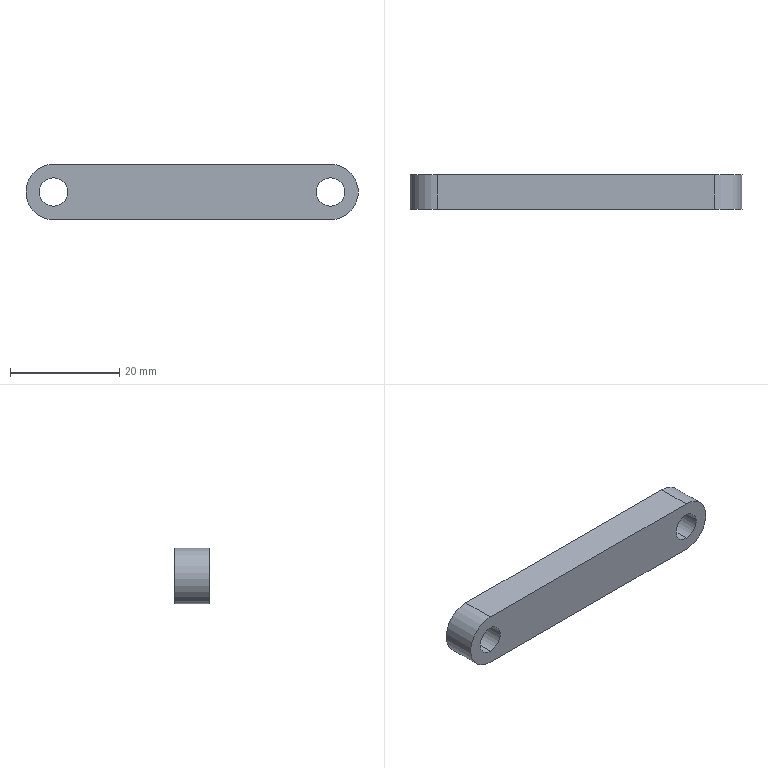Part | SolidWorks | features Extrusion 1, ICE 1 | 1 solid | 10 faces | box 60.96 x 6.35 x 10.16 mm | volume 3522 mm3 | cylinder 6 | plane 4 | commonest cylinder face diameters 5.207 x4 10.16 x2
STEP:
#1=CARTESIAN_POINT('',(50.8,0.,-2.604));
#2=VERTEX_POINT('',#1);
#3=CARTESIAN_POINT('',(50.8,0.,2.604));
#4=VERTEX_POINT('',#3);
#5=CARTESIAN_POINT('',(50.8,0.,0.));
#6=DIRECTION('',(0.,1.,0.));
#7=DIRECTION('',(0.,0.,-1.));
#8=AXIS2_PLACEMENT_3D('',#5,#6,#7);
#9=CIRCLE('',#8,2.604);
#10=EDGE_CURVE('',#2,#4,#9,.T.);
#11=ORIENTED_EDGE('',*,*,#10,.F.);
#12=CARTESIAN_POINT('',(50.8,6.35,-2.604));
#13=VERTEX_POINT('',#12);
#14=CARTESIAN_POINT('',(50.8,-8.202,-2.604));
#15=DIRECTION('',(0.,1.,0.));
#16=VECTOR('',#15,1000.);
#17=LINE('',#14,#16);
#18=EDGE_CURVE('',#2,#13,#17,.T.);
#19=ORIENTED_EDGE('',*,*,#18,.T.);
#20=CARTESIAN_POINT('',(50.8,6.35,2.604));
#21=VERTEX_POINT('',#20);
#22=CARTESIAN_POINT('',(50.8,6.35,0.));
#23=DIRECTION('',(0.,1.,0.));
#24=DIRECTION('',(0.,0.,1.));
#25=AXIS2_PLACEMENT_3D('',#22,#23,#24);
#26=CIRCLE('',#25,2.604);
#27=EDGE_CURVE('',#13,#21,#26,.T.);
#28=ORIENTED_EDGE('',*,*,#27,.T.);
#29=CARTESIAN_POINT('',(50.8,-8.202,2.604));
#30=DIRECTION('',(0.,1.,0.));
#31=VECTOR('',#30,1000.);
#32=LINE('',#29,#31);
#33=EDGE_CURVE('',#4,#21,#32,.T.);
#34=ORIENTED_EDGE('',*,*,#33,.F.);
#35=EDGE_LOOP('',(#11,#19,#28,#34));
#36=FACE_OUTER_BOUND('',#35,.T.);
#37=CARTESIAN_POINT('',(50.8,-8.202,0.));
#38=DIRECTION('',(0.,1.,0.));
#39=DIRECTION('',(0.,0.,1.));
#40=AXIS2_PLACEMENT_3D('',#37,#38,#39);
#41=CYLINDRICAL_SURFACE('',#40,2.604);
#42=ADVANCED_FACE('',(#36),#41,.F.);
#43=CARTESIAN_POINT('',(0.,0.,-2.603));
#44=VERTEX_POINT('',#43);
#45=CARTESIAN_POINT('',(0.,0.,2.603));
#46=VERTEX_POINT('',#45);
#47=CARTESIAN_POINT('',(0.,0.,0.));
#48=DIRECTION('',(0.,1.,0.));
#49=DIRECTION('',(0.,0.,-1.));
#50=AXIS2_PLACEMENT_3D('',#47,#48,#49);
#51=CIRCLE('',#50,2.603);
#52=EDGE_CURVE('',#44,#46,#51,.T.);
#53=ORIENTED_EDGE('',*,*,#52,.F.);
#54=CARTESIAN_POINT('',(0.,6.35,-2.603));
#55=VERTEX_POINT('',#54);
#56=CARTESIAN_POINT('',(0.,-8.202,-2.603));
#57=DIRECTION('',(0.,1.,0.));
#58=VECTOR('',#57,1000.);
#59=LINE('',#56,#58);
#60=EDGE_CURVE('',#44,#55,#59,.T.);
#61=ORIENTED_EDGE('',*,*,#60,.T.);
#62=CARTESIAN_POINT('',(0.,6.35,2.603));
#63=VERTEX_POINT('',#62);
#64=CARTESIAN_POINT('',(0.,6.35,0.));
#65=DIRECTION('',(0.,1.,0.));
#66=DIRECTION('',(0.,0.,1.));
#67=AXIS2_PLACEMENT_3D('',#64,#65,#66);
#68=CIRCLE('',#67,2.603);
#69=EDGE_CURVE('',#55,#63,#68,.T.);
#70=ORIENTED_EDGE('',*,*,#69,.T.);
#71=CARTESIAN_POINT('',(0.,-8.202,2.603));
#72=DIRECTION('',(0.,1.,0.));
#73=VECTOR('',#72,1000.);
#74=LINE('',#71,#73);
#75=EDGE_CURVE('',#46,#63,#74,.T.);
#76=ORIENTED_EDGE('',*,*,#75,.F.);
#77=EDGE_LOOP('',(#53,#61,#70,#76));
#78=FACE_OUTER_BOUND('',#77,.T.);
#79=CARTESIAN_POINT('',(0.,-8.202,0.));
#80=DIRECTION('',(0.,1.,0.));
#81=DIRECTION('',(0.,0.,1.));
#82=AXIS2_PLACEMENT_3D('',#79,#80,#81);
#83=CYLINDRICAL_SURFACE('',#82,2.603);
#84=ADVANCED_FACE('',(#78),#83,.F.);
#85=CARTESIAN_POINT('',(0.,6.35,-5.08));
#86=VERTEX_POINT('',#85);
#87=CARTESIAN_POINT('',(0.,6.35,5.08));
#88=VERTEX_POINT('',#87);
#89=CARTESIAN_POINT('',(0.,6.35,0.));
#90=DIRECTION('',(0.,1.,0.));
#91=DIRECTION('',(0.,0.,-1.));
#92=AXIS2_PLACEMENT_3D('',#89,#90,#91);
#93=CIRCLE('',#92,5.08);
#94=EDGE_CURVE('',#86,#88,#93,.T.);
#95=ORIENTED_EDGE('',*,*,#94,.T.);
#96=CARTESIAN_POINT('',(50.8,6.35,5.08));
#97=VERTEX_POINT('',#96);
#98=CARTESIAN_POINT('',(0.,6.35,5.08));
#99=DIRECTION('',(1.,0.,0.));
#100=VECTOR('',#99,1000.);
#101=LINE('',#98,#100);
#102=EDGE_CURVE('',#88,#97,#101,.T.);
#103=ORIENTED_EDGE('',*,*,#102,.T.);
#104=CARTESIAN_POINT('',(50.8,6.35,-5.08));
#105=VERTEX_POINT('',#104);
#106=CARTESIAN_POINT('',(50.8,6.35,0.));
#107=DIRECTION('',(0.,1.,0.));
#108=DIRECTION('',(0.,0.,-1.));
#109=AXIS2_PLACEMENT_3D('',#106,#107,#108);
#110=CIRCLE('',#109,5.08);
#111=EDGE_CURVE('',#97,#105,#110,.T.);
#112=ORIENTED_EDGE('',*,*,#111,.T.);
#113=CARTESIAN_POINT('',(0.,6.35,-5.08));
#114=DIRECTION('',(-1.,0.,0.));
#115=VECTOR('',#114,1000.);
#116=LINE('',#113,#115);
#117=EDGE_CURVE('',#105,#86,#116,.T.);
#118=ORIENTED_EDGE('',*,*,#117,.T.);
#119=EDGE_LOOP('',(#95,#103,#112,#118));
#120=FACE_OUTER_BOUND('',#119,.T.);
#121=CARTESIAN_POINT('',(0.,6.35,0.));
#122=DIRECTION('',(0.,1.,0.));
#123=DIRECTION('',(0.,0.,1.));
#124=AXIS2_PLACEMENT_3D('',#121,#122,#123);
#125=CIRCLE('',#124,2.603);
#126=EDGE_CURVE('',#63,#55,#125,.T.);
#127=ORIENTED_EDGE('',*,*,#126,.F.);
#128=ORIENTED_EDGE('',*,*,#69,.F.);
#129=EDGE_LOOP('',(#127,#128));
#130=FACE_BOUND('',#129,.T.);
#131=CARTESIAN_POINT('',(50.8,6.35,0.));
#132=DIRECTION('',(0.,1.,0.));
#133=DIRECTION('',(0.,0.,1.));
#134=AXIS2_PLACEMENT_3D('',#131,#132,#133);
#135=CIRCLE('',#134,2.604);
#136=EDGE_CURVE('',#21,#13,#135,.T.);
#137=ORIENTED_EDGE('',*,*,#136,.F.);
#138=ORIENTED_EDGE('',*,*,#27,.F.);
#139=EDGE_LOOP('',(#137,#138));
#140=FACE_BOUND('',#139,.T.);
#141=CARTESIAN_POINT('',(0.,6.35,0.));
#142=DIRECTION('',(0.,-1.,0.));
#143=DIRECTION('',(0.,0.,-1.));
#144=AXIS2_PLACEMENT_3D('',#141,#142,#143);
#145=PLANE('',#144);
#146=ADVANCED_FACE('',(#120,#130,#140),#145,.F.);
#147=CARTESIAN_POINT('',(0.,0.,-5.08));
#148=VERTEX_POINT('',#147);
#149=CARTESIAN_POINT('',(0.,0.,5.08));
#150=VERTEX_POINT('',#149);
#151=CARTESIAN_POINT('',(0.,0.,0.));
#152=DIRECTION('',(0.,1.,0.));
#153=DIRECTION('',(0.,0.,-1.));
#154=AXIS2_PLACEMENT_3D('',#151,#152,#153);
#155=CIRCLE('',#154,5.08);
#156=EDGE_CURVE('',#148,#150,#155,.T.);
#157=ORIENTED_EDGE('',*,*,#156,.F.);
#158=CARTESIAN_POINT('',(50.8,0.,-5.08));
#159=VERTEX_POINT('',#158);
#160=CARTESIAN_POINT('',(0.,0.,-5.08));
#161=DIRECTION('',(-1.,0.,0.));
#162=VECTOR('',#161,1000.);
#163=LINE('',#160,#162);
#164=EDGE_CURVE('',#159,#148,#163,.T.);
#165=ORIENTED_EDGE('',*,*,#164,.F.);
#166=CARTESIAN_POINT('',(50.8,0.,5.08));
#167=VERTEX_POINT('',#166);
#168=CARTESIAN_POINT('',(50.8,0.,0.));
#169=DIRECTION('',(0.,1.,0.));
#170=DIRECTION('',(0.,0.,-1.));
#171=AXIS2_PLACEMENT_3D('',#168,#169,#170);
#172=CIRCLE('',#171,5.08);
#173=EDGE_CURVE('',#167,#159,#172,.T.);
#174=ORIENTED_EDGE('',*,*,#173,.F.);
#175=CARTESIAN_POINT('',(0.,0.,5.08));
#176=DIRECTION('',(1.,0.,0.));
#177=VECTOR('',#176,1000.);
#178=LINE('',#175,#177);
#179=EDGE_CURVE('',#150,#167,#178,.T.);
#180=ORIENTED_EDGE('',*,*,#179,.F.);
#181=EDGE_LOOP('',(#157,#165,#174,#180));
#182=FACE_OUTER_BOUND('',#181,.T.);
#183=CARTESIAN_POINT('',(0.,0.,0.));
#184=DIRECTION('',(0.,1.,0.));
#185=DIRECTION('',(0.,0.,-1.));
#186=AXIS2_PLACEMENT_3D('',#183,#184,#185);
#187=CIRCLE('',#186,2.603);
#188=EDGE_CURVE('',#46,#44,#187,.T.);
#189=ORIENTED_EDGE('',*,*,#188,.T.);
#190=ORIENTED_EDGE('',*,*,#52,.T.);
#191=EDGE_LOOP('',(#189,#190));
#192=FACE_BOUND('',#191,.T.);
#193=CARTESIAN_POINT('',(50.8,0.,0.));
#194=DIRECTION('',(0.,1.,0.));
#195=DIRECTION('',(0.,0.,-1.));
#196=AXIS2_PLACEMENT_3D('',#193,#194,#195);
#197=CIRCLE('',#196,2.604);
#198=EDGE_CURVE('',#4,#2,#197,.T.);
#199=ORIENTED_EDGE('',*,*,#198,.T.);
#200=ORIENTED_EDGE('',*,*,#10,.T.);
#201=EDGE_LOOP('',(#199,#200));
#202=FACE_BOUND('',#201,.T.);
#203=CARTESIAN_POINT('',(0.,0.,0.));
#204=DIRECTION('',(0.,-1.,0.));
#205=DIRECTION('',(0.,0.,-1.));
#206=AXIS2_PLACEMENT_3D('',#203,#204,#205);
#207=PLANE('',#206);
#208=ADVANCED_FACE('',(#182,#192,#202),#207,.T.);
#209=ORIENTED_EDGE('',*,*,#156,.T.);
#210=CARTESIAN_POINT('',(0.,6.35,5.08));
#211=DIRECTION('',(0.,-1.,0.));
#212=VECTOR('',#211,1000.);
#213=LINE('',#210,#212);
#214=EDGE_CURVE('',#88,#150,#213,.T.);
#215=ORIENTED_EDGE('',*,*,#214,.F.);
#216=ORIENTED_EDGE('',*,*,#94,.F.);
#217=CARTESIAN_POINT('',(0.,6.35,-5.08));
#218=DIRECTION('',(0.,-1.,0.));
#219=VECTOR('',#218,1000.);
#220=LINE('',#217,#219);
#221=EDGE_CURVE('',#86,#148,#220,.T.);
#222=ORIENTED_EDGE('',*,*,#221,.T.);
#223=EDGE_LOOP('',(#209,#215,#216,#222));
#224=FACE_OUTER_BOUND('',#223,.T.);
#225=CARTESIAN_POINT('',(0.,6.35,0.));
#226=DIRECTION('',(0.,-1.,0.));
#227=DIRECTION('',(0.,0.,-1.));
#228=AXIS2_PLACEMENT_3D('',#225,#226,#227);
#229=CYLINDRICAL_SURFACE('',#228,5.08);
#230=ADVANCED_FACE('',(#224),#229,.T.);
#231=ORIENTED_EDGE('',*,*,#179,.T.);
#232=CARTESIAN_POINT('',(50.8,6.35,5.08));
#233=DIRECTION('',(0.,-1.,0.));
#234=VECTOR('',#233,1000.);
#235=LINE('',#232,#234);
#236=EDGE_CURVE('',#97,#167,#235,.T.);
#237=ORIENTED_EDGE('',*,*,#236,.F.);
#238=ORIENTED_EDGE('',*,*,#102,.F.);
#239=ORIENTED_EDGE('',*,*,#214,.T.);
#240=EDGE_LOOP('',(#231,#237,#238,#239));
#241=FACE_OUTER_BOUND('',#240,.T.);
#242=CARTESIAN_POINT('',(0.,6.35,5.08));
#243=DIRECTION('',(0.,0.,-1.));
#244=DIRECTION('',(-1.,0.,0.));
#245=AXIS2_PLACEMENT_3D('',#242,#243,#244);
#246=PLANE('',#245);
#247=ADVANCED_FACE('',(#241),#246,.F.);
#248=ORIENTED_EDGE('',*,*,#173,.T.);
#249=CARTESIAN_POINT('',(50.8,6.35,-5.08));
#250=DIRECTION('',(0.,-1.,0.));
#251=VECTOR('',#250,1000.);
#252=LINE('',#249,#251);
#253=EDGE_CURVE('',#105,#159,#252,.T.);
#254=ORIENTED_EDGE('',*,*,#253,.F.);
#255=ORIENTED_EDGE('',*,*,#111,.F.);
#256=ORIENTED_EDGE('',*,*,#236,.T.);
#257=EDGE_LOOP('',(#248,#254,#255,#256));
#258=FACE_OUTER_BOUND('',#257,.T.);
#259=CARTESIAN_POINT('',(50.8,6.35,0.));
#260=DIRECTION('',(0.,-1.,0.));
#261=DIRECTION('',(0.,0.,-1.));
#262=AXIS2_PLACEMENT_3D('',#259,#260,#261);
#263=CYLINDRICAL_SURFACE('',#262,5.08);
#264=ADVANCED_FACE('',(#258),#263,.T.);
#265=ORIENTED_EDGE('',*,*,#164,.T.);
#266=ORIENTED_EDGE('',*,*,#221,.F.);
#267=ORIENTED_EDGE('',*,*,#117,.F.);
#268=ORIENTED_EDGE('',*,*,#253,.T.);
#269=EDGE_LOOP('',(#265,#266,#267,#268));
#270=FACE_OUTER_BOUND('',#269,.T.);
#271=CARTESIAN_POINT('',(0.,6.35,-5.08));
#272=DIRECTION('',(0.,0.,1.));
#273=DIRECTION('',(1.,0.,0.));
#274=AXIS2_PLACEMENT_3D('',#271,#272,#273);
#275=PLANE('',#274);
#276=ADVANCED_FACE('',(#270),#275,.F.);
#277=ORIENTED_EDGE('',*,*,#60,.F.);
#278=ORIENTED_EDGE('',*,*,#188,.F.);
#279=ORIENTED_EDGE('',*,*,#75,.T.);
#280=ORIENTED_EDGE('',*,*,#126,.T.);
#281=EDGE_LOOP('',(#277,#278,#279,#280));
#282=FACE_OUTER_BOUND('',#281,.T.);
#283=CARTESIAN_POINT('',(0.,-8.202,0.));
#284=DIRECTION('',(0.,1.,0.));
#285=DIRECTION('',(0.,0.,1.));
#286=AXIS2_PLACEMENT_3D('',#283,#284,#285);
#287=CYLINDRICAL_SURFACE('',#286,2.603);
#288=ADVANCED_FACE('',(#282),#287,.F.);
#289=ORIENTED_EDGE('',*,*,#18,.F.);
#290=ORIENTED_EDGE('',*,*,#198,.F.);
#291=ORIENTED_EDGE('',*,*,#33,.T.);
#292=ORIENTED_EDGE('',*,*,#136,.T.);
#293=EDGE_LOOP('',(#289,#290,#291,#292));
#294=FACE_OUTER_BOUND('',#293,.T.);
#295=CARTESIAN_POINT('',(50.8,-8.202,0.));
#296=DIRECTION('',(0.,1.,0.));
#297=DIRECTION('',(0.,0.,1.));
#298=AXIS2_PLACEMENT_3D('',#295,#296,#297);
#299=CYLINDRICAL_SURFACE('',#298,2.604);
#300=ADVANCED_FACE('',(#294),#299,.F.);
#301=CLOSED_SHELL('',(#42,#84,#146,#208,#230,#247,#264,#276,#288,#300));
#302=MANIFOLD_SOLID_BREP('',#301);
#303=CARTESIAN_POINT('',(0.,0.,0.));
#304=DIRECTION('',(0.,0.,1.));
#305=DIRECTION('',(1.,0.,0.));
#306=AXIS2_PLACEMENT_3D('',#303,#304,#305);
#307=(LENGTH_UNIT()NAMED_UNIT(*)SI_UNIT(.MILLI.,.METRE.));
#308=UNCERTAINTY_MEASURE_WITH_UNIT(LENGTH_MEASURE(0.00001),#307,'','');
#309=(NAMED_UNIT(*)PLANE_ANGLE_UNIT()SI_UNIT($,.RADIAN.));
#310=(NAMED_UNIT(*)SI_UNIT($,.STERADIAN.)SOLID_ANGLE_UNIT());
#311=(GEOMETRIC_REPRESENTATION_CONTEXT(3)GLOBAL_UNCERTAINTY_ASSIGNED_CONTEXT((#308))GLOBAL_UNIT_ASSIGNED_CONTEXT((#307,#309,#310))REPRESENTATION_CONTEXT('',''));
#312=ADVANCED_BREP_SHAPE_REPRESENTATION('',(#302,#306),#311);